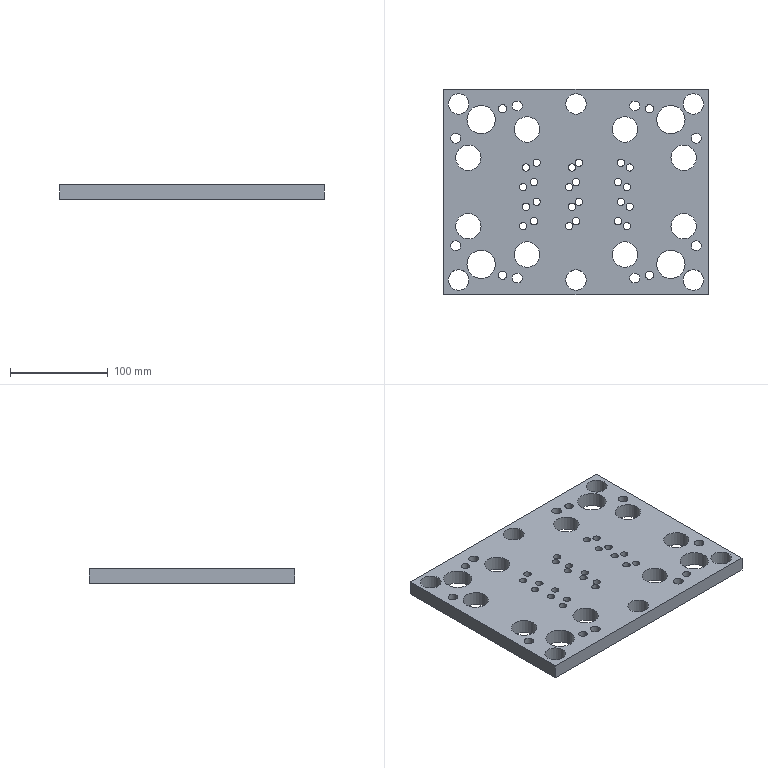Part | STEP file | 1 solid | 63 faces | box 270 x 210 x 15 mm | volume 687226 mm3 | cylinder 54 | plane 6 | cone 3 | commonest cylinder face diameters 7.5 x24 10 x8 26 x8 21 x6 8.5 x4 29 x4